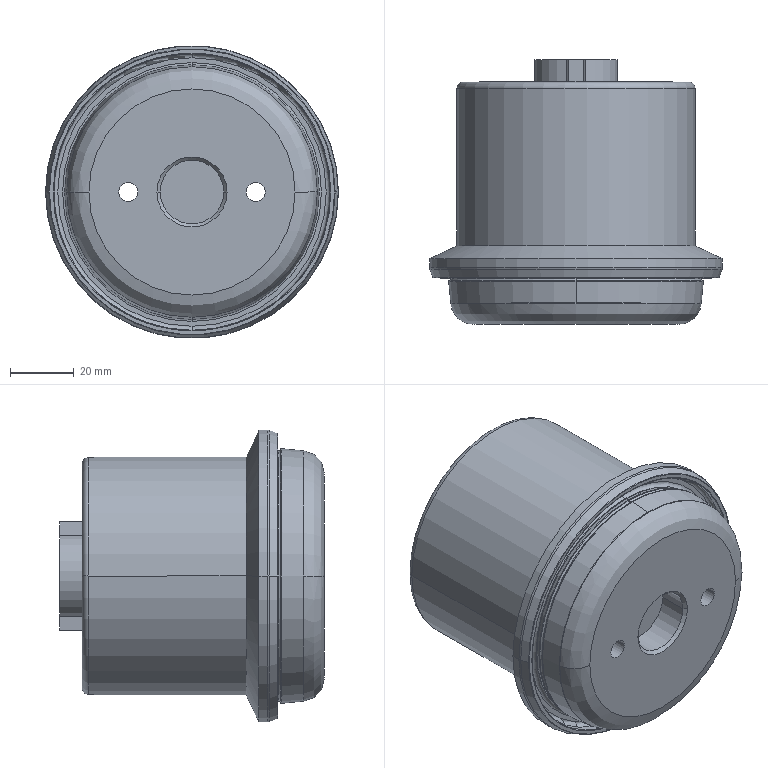Part | SolidWorks | features Fillet 7, ICE 5, Chamfer 3, RevCut 3, CirPattern 1, Revolution 1 | 1 solid | 75 faces | box 92 x 83 x 92 mm | volume 147042 mm3 | torus 26 | cylinder 18 | cone 16 | plane 15 | commonest cylinder face diameters 6 x4 20 x4 16 x2 26 x2 74.8 x2 86.8 x2